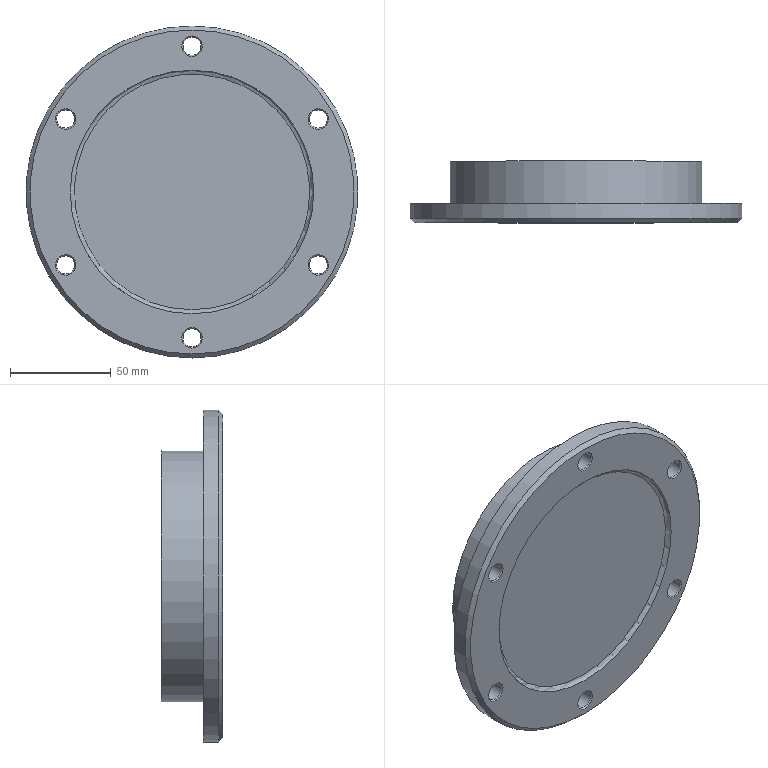Part | NX | 1 solid | 29 faces | box 165 x 30.6 x 165 mm | volume 264298 mm3 | cone 14 | cylinder 8 | plane 5 | torus 2 | commonest cylinder face diameters 9 x6 125 x1 165 x1
STEP:
#1=CARTESIAN_POINT('',(69.093,93.861,38.5));
#2=VERTEX_POINT('',#1);
#3=CARTESIAN_POINT('',(65.196,93.861,36.25));
#4=DIRECTION('',(0.,-1.,0.));
#5=DIRECTION('',(0.866,0.,0.5));
#6=AXIS2_PLACEMENT_3D('',#3,#4,#5);
#7=CIRCLE('',#6,4.5);
#8=EDGE_CURVE('',#2,#2,#7,.T.);
#9=ORIENTED_EDGE('',*,*,#8,.F.);
#10=EDGE_LOOP('',(#9));
#11=FACE_BOUND('',#10,.T.);
#12=CARTESIAN_POINT('',(69.612,93.261,38.8));
#13=VERTEX_POINT('',#12);
#14=CARTESIAN_POINT('',(65.196,93.261,36.25));
#15=DIRECTION('',(0.,1.,0.));
#16=DIRECTION('',(0.866,0.,0.5));
#17=AXIS2_PLACEMENT_3D('',#14,#15,#16);
#18=CIRCLE('',#17,5.1);
#19=EDGE_CURVE('',#13,#13,#18,.T.);
#20=ORIENTED_EDGE('',*,*,#19,.F.);
#21=EDGE_LOOP('',(#20));
#22=FACE_BOUND('',#21,.T.);
#23=CARTESIAN_POINT('',(65.196,93.261,36.25));
#24=DIRECTION('',(0.,-1.,0.));
#25=DIRECTION('',(0.866,0.,0.5));
#26=AXIS2_PLACEMENT_3D('',#23,#24,#25);
#27=CONICAL_SURFACE('',#26,5.1,45.);
#28=ADVANCED_FACE('',(#11,#22),#27,.F.);
#29=CARTESIAN_POINT('',(61.298,102.261,34.));
#30=VERTEX_POINT('',#29);
#31=CARTESIAN_POINT('',(65.196,102.261,36.25));
#32=DIRECTION('',(0.,1.,0.));
#33=DIRECTION('',(-0.866,0.,-0.5));
#34=AXIS2_PLACEMENT_3D('',#31,#32,#33);
#35=CIRCLE('',#34,4.5);
#36=EDGE_CURVE('',#30,#30,#35,.T.);
#37=ORIENTED_EDGE('',*,*,#36,.F.);
#38=EDGE_LOOP('',(#37));
#39=FACE_BOUND('',#38,.T.);
#40=CARTESIAN_POINT('',(60.779,102.861,33.7));
#41=VERTEX_POINT('',#40);
#42=CARTESIAN_POINT('',(65.196,102.861,36.25));
#43=DIRECTION('',(0.,-1.,0.));
#44=DIRECTION('',(-0.866,0.,-0.5));
#45=AXIS2_PLACEMENT_3D('',#42,#43,#44);
#46=CIRCLE('',#45,5.1);
#47=EDGE_CURVE('',#41,#41,#46,.T.);
#48=ORIENTED_EDGE('',*,*,#47,.F.);
#49=EDGE_LOOP('',(#48));
#50=FACE_BOUND('',#49,.T.);
#51=CARTESIAN_POINT('',(65.196,102.861,36.25));
#52=DIRECTION('',(0.,1.,0.));
#53=DIRECTION('',(-0.866,0.,-0.5));
#54=AXIS2_PLACEMENT_3D('',#51,#52,#53);
#55=CONICAL_SURFACE('',#54,5.1,45.);
#56=ADVANCED_FACE('',(#39,#50),#55,.F.);
#57=ORIENTED_EDGE('',*,*,#36,.T.);
#58=EDGE_LOOP('',(#57));
#59=FACE_BOUND('',#58,.T.);
#60=ORIENTED_EDGE('',*,*,#8,.T.);
#61=EDGE_LOOP('',(#60));
#62=FACE_BOUND('',#61,.T.);
#63=CARTESIAN_POINT('',(65.196,93.261,36.25));
#64=DIRECTION('',(0.,1.,0.));
#65=DIRECTION('',(-0.866,0.,-0.5));
#66=AXIS2_PLACEMENT_3D('',#63,#64,#65);
#67=CYLINDRICAL_SURFACE('',#66,4.5);
#68=ADVANCED_FACE('',(#59,#62),#67,.F.);
#69=CARTESIAN_POINT('',(69.093,93.861,-38.5));
#70=VERTEX_POINT('',#69);
#71=CARTESIAN_POINT('',(65.196,93.861,-36.25));
#72=DIRECTION('',(0.,-1.,0.));
#73=DIRECTION('',(0.866,0.,-0.5));
#74=AXIS2_PLACEMENT_3D('',#71,#72,#73);
#75=CIRCLE('',#74,4.5);
#76=EDGE_CURVE('',#70,#70,#75,.T.);
#77=ORIENTED_EDGE('',*,*,#76,.F.);
#78=EDGE_LOOP('',(#77));
#79=FACE_BOUND('',#78,.T.);
#80=CARTESIAN_POINT('',(69.612,93.261,-38.8));
#81=VERTEX_POINT('',#80);
#82=CARTESIAN_POINT('',(65.196,93.261,-36.25));
#83=DIRECTION('',(0.,1.,0.));
#84=DIRECTION('',(0.866,0.,-0.5));
#85=AXIS2_PLACEMENT_3D('',#82,#83,#84);
#86=CIRCLE('',#85,5.1);
#87=EDGE_CURVE('',#81,#81,#86,.T.);
#88=ORIENTED_EDGE('',*,*,#87,.F.);
#89=EDGE_LOOP('',(#88));
#90=FACE_BOUND('',#89,.T.);
#91=CARTESIAN_POINT('',(65.196,93.261,-36.25));
#92=DIRECTION('',(0.,-1.,0.));
#93=DIRECTION('',(0.866,0.,-0.5));
#94=AXIS2_PLACEMENT_3D('',#91,#92,#93);
#95=CONICAL_SURFACE('',#94,5.1,45.);
#96=ADVANCED_FACE('',(#79,#90),#95,.F.);
#97=CARTESIAN_POINT('',(61.298,102.261,-34.));
#98=VERTEX_POINT('',#97);
#99=CARTESIAN_POINT('',(65.196,102.261,-36.25));
#100=DIRECTION('',(0.,1.,0.));
#101=DIRECTION('',(-0.866,0.,0.5));
#102=AXIS2_PLACEMENT_3D('',#99,#100,#101);
#103=CIRCLE('',#102,4.5);
#104=EDGE_CURVE('',#98,#98,#103,.T.);
#105=ORIENTED_EDGE('',*,*,#104,.F.);
#106=EDGE_LOOP('',(#105));
#107=FACE_BOUND('',#106,.T.);
#108=CARTESIAN_POINT('',(60.779,102.861,-33.7));
#109=VERTEX_POINT('',#108);
#110=CARTESIAN_POINT('',(65.196,102.861,-36.25));
#111=DIRECTION('',(0.,-1.,0.));
#112=DIRECTION('',(-0.866,0.,0.5));
#113=AXIS2_PLACEMENT_3D('',#110,#111,#112);
#114=CIRCLE('',#113,5.1);
#115=EDGE_CURVE('',#109,#109,#114,.T.);
#116=ORIENTED_EDGE('',*,*,#115,.F.);
#117=EDGE_LOOP('',(#116));
#118=FACE_BOUND('',#117,.T.);
#119=CARTESIAN_POINT('',(65.196,102.861,-36.25));
#120=DIRECTION('',(0.,1.,0.));
#121=DIRECTION('',(-0.866,0.,0.5));
#122=AXIS2_PLACEMENT_3D('',#119,#120,#121);
#123=CONICAL_SURFACE('',#122,5.1,45.);
#124=ADVANCED_FACE('',(#107,#118),#123,.F.);
#125=ORIENTED_EDGE('',*,*,#104,.T.);
#126=EDGE_LOOP('',(#125));
#127=FACE_BOUND('',#126,.T.);
#128=ORIENTED_EDGE('',*,*,#76,.T.);
#129=EDGE_LOOP('',(#128));
#130=FACE_BOUND('',#129,.T.);
#131=CARTESIAN_POINT('',(65.196,93.261,-36.25));
#132=DIRECTION('',(0.,1.,0.));
#133=DIRECTION('',(-0.866,0.,0.5));
#134=AXIS2_PLACEMENT_3D('',#131,#132,#133);
#135=CYLINDRICAL_SURFACE('',#134,4.5);
#136=ADVANCED_FACE('',(#127,#130),#135,.F.);
#137=CARTESIAN_POINT('',(2.409,93.861,-77.));
#138=VERTEX_POINT('',#137);
#139=CARTESIAN_POINT('',(2.409,93.861,-72.5));
#140=DIRECTION('',(0.,-1.,0.));
#141=DIRECTION('',(0.,0.,-1.));
#142=AXIS2_PLACEMENT_3D('',#139,#140,#141);
#143=CIRCLE('',#142,4.5);
#144=EDGE_CURVE('',#138,#138,#143,.T.);
#145=ORIENTED_EDGE('',*,*,#144,.F.);
#146=EDGE_LOOP('',(#145));
#147=FACE_BOUND('',#146,.T.);
#148=CARTESIAN_POINT('',(2.409,93.261,-77.6));
#149=VERTEX_POINT('',#148);
#150=CARTESIAN_POINT('',(2.409,93.261,-72.5));
#151=DIRECTION('',(0.,1.,0.));
#152=DIRECTION('',(0.,0.,-1.));
#153=AXIS2_PLACEMENT_3D('',#150,#151,#152);
#154=CIRCLE('',#153,5.1);
#155=EDGE_CURVE('',#149,#149,#154,.T.);
#156=ORIENTED_EDGE('',*,*,#155,.F.);
#157=EDGE_LOOP('',(#156));
#158=FACE_BOUND('',#157,.T.);
#159=CARTESIAN_POINT('',(2.409,93.261,-72.5));
#160=DIRECTION('',(0.,-1.,0.));
#161=DIRECTION('',(0.,0.,-1.));
#162=AXIS2_PLACEMENT_3D('',#159,#160,#161);
#163=CONICAL_SURFACE('',#162,5.1,45.);
#164=ADVANCED_FACE('',(#147,#158),#163,.F.);
#165=CARTESIAN_POINT('',(2.409,102.261,-68.));
#166=VERTEX_POINT('',#165);
#167=CARTESIAN_POINT('',(2.409,102.261,-72.5));
#168=DIRECTION('',(0.,1.,0.));
#169=DIRECTION('',(0.,0.,1.));
#170=AXIS2_PLACEMENT_3D('',#167,#168,#169);
#171=CIRCLE('',#170,4.5);
#172=EDGE_CURVE('',#166,#166,#171,.T.);
#173=ORIENTED_EDGE('',*,*,#172,.F.);
#174=EDGE_LOOP('',(#173));
#175=FACE_BOUND('',#174,.T.);
#176=CARTESIAN_POINT('',(2.409,102.861,-67.4));
#177=VERTEX_POINT('',#176);
#178=CARTESIAN_POINT('',(2.409,102.861,-72.5));
#179=DIRECTION('',(0.,-1.,0.));
#180=DIRECTION('',(0.,0.,1.));
#181=AXIS2_PLACEMENT_3D('',#178,#179,#180);
#182=CIRCLE('',#181,5.1);
#183=EDGE_CURVE('',#177,#177,#182,.T.);
#184=ORIENTED_EDGE('',*,*,#183,.F.);
#185=EDGE_LOOP('',(#184));
#186=FACE_BOUND('',#185,.T.);
#187=CARTESIAN_POINT('',(2.409,102.861,-72.5));
#188=DIRECTION('',(0.,1.,0.));
#189=DIRECTION('',(0.,0.,1.));
#190=AXIS2_PLACEMENT_3D('',#187,#188,#189);
#191=CONICAL_SURFACE('',#190,5.1,45.);
#192=ADVANCED_FACE('',(#175,#186),#191,.F.);
#193=ORIENTED_EDGE('',*,*,#172,.T.);
#194=EDGE_LOOP('',(#193));
#195=FACE_BOUND('',#194,.T.);
#196=ORIENTED_EDGE('',*,*,#144,.T.);
#197=EDGE_LOOP('',(#196));
#198=FACE_BOUND('',#197,.T.);
#199=CARTESIAN_POINT('',(2.409,93.261,-72.5));
#200=DIRECTION('',(0.,1.,0.));
#201=DIRECTION('',(0.,0.,1.));
#202=AXIS2_PLACEMENT_3D('',#199,#200,#201);
#203=CYLINDRICAL_SURFACE('',#202,4.5);
#204=ADVANCED_FACE('',(#195,#198),#203,.F.);
#205=CARTESIAN_POINT('',(-64.275,93.861,-38.5));
#206=VERTEX_POINT('',#205);
#207=CARTESIAN_POINT('',(-60.378,93.861,-36.25));
#208=DIRECTION('',(0.,-1.,0.));
#209=DIRECTION('',(-0.866,0.,-0.5));
#210=AXIS2_PLACEMENT_3D('',#207,#208,#209);
#211=CIRCLE('',#210,4.5);
#212=EDGE_CURVE('',#206,#206,#211,.T.);
#213=ORIENTED_EDGE('',*,*,#212,.F.);
#214=EDGE_LOOP('',(#213));
#215=FACE_BOUND('',#214,.T.);
#216=CARTESIAN_POINT('',(-64.795,93.261,-38.8));
#217=VERTEX_POINT('',#216);
#218=CARTESIAN_POINT('',(-60.378,93.261,-36.25));
#219=DIRECTION('',(0.,1.,0.));
#220=DIRECTION('',(-0.866,0.,-0.5));
#221=AXIS2_PLACEMENT_3D('',#218,#219,#220);
#222=CIRCLE('',#221,5.1);
#223=EDGE_CURVE('',#217,#217,#222,.T.);
#224=ORIENTED_EDGE('',*,*,#223,.F.);
#225=EDGE_LOOP('',(#224));
#226=FACE_BOUND('',#225,.T.);
#227=CARTESIAN_POINT('',(-60.378,93.261,-36.25));
#228=DIRECTION('',(0.,-1.,0.));
#229=DIRECTION('',(-0.866,0.,-0.5));
#230=AXIS2_PLACEMENT_3D('',#227,#228,#229);
#231=CONICAL_SURFACE('',#230,5.1,45.);
#232=ADVANCED_FACE('',(#215,#226),#231,.F.);
#233=CARTESIAN_POINT('',(-56.481,102.261,-34.));
#234=VERTEX_POINT('',#233);
#235=CARTESIAN_POINT('',(-60.378,102.261,-36.25));
#236=DIRECTION('',(0.,1.,0.));
#237=DIRECTION('',(0.866,0.,0.5));
#238=AXIS2_PLACEMENT_3D('',#235,#236,#237);
#239=CIRCLE('',#238,4.5);
#240=EDGE_CURVE('',#234,#234,#239,.T.);
#241=ORIENTED_EDGE('',*,*,#240,.F.);
#242=EDGE_LOOP('',(#241));
#243=FACE_BOUND('',#242,.T.);
#244=CARTESIAN_POINT('',(-55.961,102.861,-33.7));
#245=VERTEX_POINT('',#244);
#246=CARTESIAN_POINT('',(-60.378,102.861,-36.25));
#247=DIRECTION('',(0.,-1.,0.));
#248=DIRECTION('',(0.866,0.,0.5));
#249=AXIS2_PLACEMENT_3D('',#246,#247,#248);
#250=CIRCLE('',#249,5.1);
#251=EDGE_CURVE('',#245,#245,#250,.T.);
#252=ORIENTED_EDGE('',*,*,#251,.F.);
#253=EDGE_LOOP('',(#252));
#254=FACE_BOUND('',#253,.T.);
#255=CARTESIAN_POINT('',(-60.378,102.861,-36.25));
#256=DIRECTION('',(0.,1.,0.));
#257=DIRECTION('',(0.866,0.,0.5));
#258=AXIS2_PLACEMENT_3D('',#255,#256,#257);
#259=CONICAL_SURFACE('',#258,5.1,45.);
#260=ADVANCED_FACE('',(#243,#254),#259,.F.);
#261=ORIENTED_EDGE('',*,*,#240,.T.);
#262=EDGE_LOOP('',(#261));
#263=FACE_BOUND('',#262,.T.);
#264=ORIENTED_EDGE('',*,*,#212,.T.);
#265=EDGE_LOOP('',(#264));
#266=FACE_BOUND('',#265,.T.);
#267=CARTESIAN_POINT('',(-60.378,93.261,-36.25));
#268=DIRECTION('',(0.,1.,0.));
#269=DIRECTION('',(0.866,0.,0.5));
#270=AXIS2_PLACEMENT_3D('',#267,#268,#269);
#271=CYLINDRICAL_SURFACE('',#270,4.5);
#272=ADVANCED_FACE('',(#263,#266),#271,.F.);
#273=CARTESIAN_POINT('',(-64.275,93.861,38.5));
#274=VERTEX_POINT('',#273);
#275=CARTESIAN_POINT('',(-60.378,93.861,36.25));
#276=DIRECTION('',(0.,-1.,0.));
#277=DIRECTION('',(-0.866,0.,0.5));
#278=AXIS2_PLACEMENT_3D('',#275,#276,#277);
#279=CIRCLE('',#278,4.5);
#280=EDGE_CURVE('',#274,#274,#279,.T.);
#281=ORIENTED_EDGE('',*,*,#280,.F.);
#282=EDGE_LOOP('',(#281));
#283=FACE_BOUND('',#282,.T.);
#284=CARTESIAN_POINT('',(-64.795,93.261,38.8));
#285=VERTEX_POINT('',#284);
#286=CARTESIAN_POINT('',(-60.378,93.261,36.25));
#287=DIRECTION('',(0.,1.,0.));
#288=DIRECTION('',(-0.866,0.,0.5));
#289=AXIS2_PLACEMENT_3D('',#286,#287,#288);
#290=CIRCLE('',#289,5.1);
#291=EDGE_CURVE('',#285,#285,#290,.T.);
#292=ORIENTED_EDGE('',*,*,#291,.F.);
#293=EDGE_LOOP('',(#292));
#294=FACE_BOUND('',#293,.T.);
#295=CARTESIAN_POINT('',(-60.378,93.261,36.25));
#296=DIRECTION('',(0.,-1.,0.));
#297=DIRECTION('',(-0.866,0.,0.5));
#298=AXIS2_PLACEMENT_3D('',#295,#296,#297);
#299=CONICAL_SURFACE('',#298,5.1,45.);
#300=ADVANCED_FACE('',(#283,#294),#299,.F.);
#301=CARTESIAN_POINT('',(-56.481,102.261,34.));
#302=VERTEX_POINT('',#301);
#303=CARTESIAN_POINT('',(-60.378,102.261,36.25));
#304=DIRECTION('',(0.,1.,0.));
#305=DIRECTION('',(0.866,0.,-0.5));
#306=AXIS2_PLACEMENT_3D('',#303,#304,#305);
#307=CIRCLE('',#306,4.5);
#308=EDGE_CURVE('',#302,#302,#307,.T.);
#309=ORIENTED_EDGE('',*,*,#308,.F.);
#310=EDGE_LOOP('',(#309));
#311=FACE_BOUND('',#310,.T.);
#312=CARTESIAN_POINT('',(-55.961,102.861,33.7));
#313=VERTEX_POINT('',#312);
#314=CARTESIAN_POINT('',(-60.378,102.861,36.25));
#315=DIRECTION('',(0.,-1.,0.));
#316=DIRECTION('',(0.866,0.,-0.5));
#317=AXIS2_PLACEMENT_3D('',#314,#315,#316);
#318=CIRCLE('',#317,5.1);
#319=EDGE_CURVE('',#313,#313,#318,.T.);
#320=ORIENTED_EDGE('',*,*,#319,.F.);
#321=EDGE_LOOP('',(#320));
#322=FACE_BOUND('',#321,.T.);
#323=CARTESIAN_POINT('',(-60.378,102.861,36.25));
#324=DIRECTION('',(0.,1.,0.));
#325=DIRECTION('',(0.866,0.,-0.5));
#326=AXIS2_PLACEMENT_3D('',#323,#324,#325);
#327=CONICAL_SURFACE('',#326,5.1,45.);
#328=ADVANCED_FACE('',(#311,#322),#327,.F.);
#329=ORIENTED_EDGE('',*,*,#308,.T.);
#330=EDGE_LOOP('',(#329));
#331=FACE_BOUND('',#330,.T.);
#332=ORIENTED_EDGE('',*,*,#280,.T.);
#333=EDGE_LOOP('',(#332));
#334=FACE_BOUND('',#333,.T.);
#335=CARTESIAN_POINT('',(-60.378,93.261,36.25));
#336=DIRECTION('',(0.,1.,0.));
#337=DIRECTION('',(0.866,0.,-0.5));
#338=AXIS2_PLACEMENT_3D('',#335,#336,#337);
#339=CYLINDRICAL_SURFACE('',#338,4.5);
#340=ADVANCED_FACE('',(#331,#334),#339,.F.);
#341=CARTESIAN_POINT('',(2.409,95.261,-58.5));
#342=VERTEX_POINT('',#341);
#343=CARTESIAN_POINT('',(2.409,95.261,0.));
#344=DIRECTION('',(0.,-1.,0.));
#345=DIRECTION('',(0.,0.,-1.));
#346=AXIS2_PLACEMENT_3D('',#343,#344,#345);
#347=CIRCLE('',#346,58.5);
#348=EDGE_CURVE('',#342,#342,#347,.T.);
#349=ORIENTED_EDGE('',*,*,#348,.T.);
#350=EDGE_LOOP('',(#349));
#351=FACE_OUTER_BOUND('',#350,.T.);
#352=CARTESIAN_POINT('',(-56.091,95.261,0.));
#353=DIRECTION('',(0.,1.,0.));
#354=DIRECTION('',(0.,0.,-1.));
#355=AXIS2_PLACEMENT_3D('',#352,#353,#354);
#356=PLANE('',#355);
#357=ADVANCED_FACE('',(#351),#356,.F.);
#358=ORIENTED_EDGE('',*,*,#348,.F.);
#359=EDGE_LOOP('',(#358));
#360=FACE_BOUND('',#359,.T.);
#361=CARTESIAN_POINT('',(2.409,93.261,-60.5));
#362=VERTEX_POINT('',#361);
#363=CARTESIAN_POINT('',(2.409,93.261,0.));
#364=DIRECTION('',(0.,-1.,0.));
#365=DIRECTION('',(0.,0.,-1.));
#366=AXIS2_PLACEMENT_3D('',#363,#364,#365);
#367=CIRCLE('',#366,60.5);
#368=EDGE_CURVE('',#362,#362,#367,.T.);
#369=ORIENTED_EDGE('',*,*,#368,.T.);
#370=EDGE_LOOP('',(#369));
#371=FACE_BOUND('',#370,.T.);
#372=CARTESIAN_POINT('',(2.409,93.261,0.));
#373=DIRECTION('',(0.,-1.,0.));
#374=DIRECTION('',(0.,0.,1.));
#375=AXIS2_PLACEMENT_3D('',#372,#373,#374);
#376=TOROIDAL_SURFACE('',#375,58.5,2.);
#377=ADVANCED_FACE('',(#360,#371),#376,.F.);
#378=ORIENTED_EDGE('',*,*,#19,.T.);
#379=EDGE_LOOP('',(#378));
#380=FACE_BOUND('',#379,.T.);
#381=ORIENTED_EDGE('',*,*,#87,.T.);
#382=EDGE_LOOP('',(#381));
#383=FACE_BOUND('',#382,.T.);
#384=ORIENTED_EDGE('',*,*,#155,.T.);
#385=EDGE_LOOP('',(#384));
#386=FACE_BOUND('',#385,.T.);
#387=ORIENTED_EDGE('',*,*,#223,.T.);
#388=EDGE_LOOP('',(#387));
#389=FACE_BOUND('',#388,.T.);
#390=ORIENTED_EDGE('',*,*,#291,.T.);
#391=EDGE_LOOP('',(#390));
#392=FACE_BOUND('',#391,.T.);
#393=CARTESIAN_POINT('',(2.409,93.261,77.6));
#394=VERTEX_POINT('',#393);
#395=CARTESIAN_POINT('',(2.409,93.261,72.5));
#396=DIRECTION('',(0.,1.,0.));
#397=DIRECTION('',(0.,0.,1.));
#398=AXIS2_PLACEMENT_3D('',#395,#396,#397);
#399=CIRCLE('',#398,5.1);
#400=EDGE_CURVE('',#394,#394,#399,.T.);
#401=ORIENTED_EDGE('',*,*,#400,.T.);
#402=EDGE_LOOP('',(#401));
#403=FACE_BOUND('',#402,.T.);
#404=ORIENTED_EDGE('',*,*,#368,.F.);
#405=EDGE_LOOP('',(#404));
#406=FACE_BOUND('',#405,.T.);
#407=CARTESIAN_POINT('',(2.409,93.261,-80.5));
#408=VERTEX_POINT('',#407);
#409=CARTESIAN_POINT('',(2.409,93.261,0.));
#410=DIRECTION('',(0.,-1.,0.));
#411=DIRECTION('',(0.,0.,-1.));
#412=AXIS2_PLACEMENT_3D('',#409,#410,#411);
#413=CIRCLE('',#412,80.5);
#414=EDGE_CURVE('',#408,#408,#413,.T.);
#415=ORIENTED_EDGE('',*,*,#414,.T.);
#416=EDGE_LOOP('',(#415));
#417=FACE_BOUND('',#416,.T.);
#418=CARTESIAN_POINT('',(-78.091,93.261,0.));
#419=DIRECTION('',(0.,1.,0.));
#420=DIRECTION('',(0.,0.,-1.));
#421=AXIS2_PLACEMENT_3D('',#418,#419,#420);
#422=PLANE('',#421);
#423=ADVANCED_FACE('',(#380,#383,#386,#389,#392,#403,#406,#417),#422,.F.);
#424=ORIENTED_EDGE('',*,*,#414,.F.);
#425=EDGE_LOOP('',(#424));
#426=FACE_BOUND('',#425,.T.);
#427=CARTESIAN_POINT('',(2.409,95.261,-82.5));
#428=VERTEX_POINT('',#427);
#429=CARTESIAN_POINT('',(2.409,95.261,0.));
#430=DIRECTION('',(0.,-1.,0.));
#431=DIRECTION('',(0.,0.,-1.));
#432=AXIS2_PLACEMENT_3D('',#429,#430,#431);
#433=CIRCLE('',#432,82.5);
#434=EDGE_CURVE('',#428,#428,#433,.T.);
#435=ORIENTED_EDGE('',*,*,#434,.T.);
#436=EDGE_LOOP('',(#435));
#437=FACE_BOUND('',#436,.T.);
#438=CARTESIAN_POINT('',(2.409,95.261,0.));
#439=DIRECTION('',(0.,1.,0.));
#440=DIRECTION('',(0.,0.,-1.));
#441=AXIS2_PLACEMENT_3D('',#438,#439,#440);
#442=CONICAL_SURFACE('',#441,82.5,45.);
#443=ADVANCED_FACE('',(#426,#437),#442,.T.);
#444=ORIENTED_EDGE('',*,*,#434,.F.);
#445=EDGE_LOOP('',(#444));
#446=FACE_BOUND('',#445,.T.);
#447=CARTESIAN_POINT('',(2.409,102.861,-82.5));
#448=VERTEX_POINT('',#447);
#449=CARTESIAN_POINT('',(2.409,102.861,0.));
#450=DIRECTION('',(0.,-1.,0.));
#451=DIRECTION('',(0.,0.,-1.));
#452=AXIS2_PLACEMENT_3D('',#449,#450,#451);
#453=CIRCLE('',#452,82.5);
#454=EDGE_CURVE('',#448,#448,#453,.T.);
#455=ORIENTED_EDGE('',*,*,#454,.T.);
#456=EDGE_LOOP('',(#455));
#457=FACE_BOUND('',#456,.T.);
#458=CARTESIAN_POINT('',(2.409,82.561,0.));
#459=DIRECTION('',(0.,-1.,0.));
#460=DIRECTION('',(0.,0.,1.));
#461=AXIS2_PLACEMENT_3D('',#458,#459,#460);
#462=CYLINDRICAL_SURFACE('',#461,82.5);
#463=ADVANCED_FACE('',(#446,#457),#462,.T.);
#464=ORIENTED_EDGE('',*,*,#47,.T.);
#465=EDGE_LOOP('',(#464));
#466=FACE_BOUND('',#465,.T.);
#467=ORIENTED_EDGE('',*,*,#115,.T.);
#468=EDGE_LOOP('',(#467));
#469=FACE_BOUND('',#468,.T.);
#470=ORIENTED_EDGE('',*,*,#183,.T.);
#471=EDGE_LOOP('',(#470));
#472=FACE_BOUND('',#471,.T.);
#473=ORIENTED_EDGE('',*,*,#251,.T.);
#474=EDGE_LOOP('',(#473));
#475=FACE_BOUND('',#474,.T.);
#476=ORIENTED_EDGE('',*,*,#319,.T.);
#477=EDGE_LOOP('',(#476));
#478=FACE_BOUND('',#477,.T.);
#479=CARTESIAN_POINT('',(2.409,102.861,67.4));
#480=VERTEX_POINT('',#479);
#481=CARTESIAN_POINT('',(2.409,102.861,72.5));
#482=DIRECTION('',(0.,-1.,0.));
#483=DIRECTION('',(0.,0.,-1.));
#484=AXIS2_PLACEMENT_3D('',#481,#482,#483);
#485=CIRCLE('',#484,5.1);
#486=EDGE_CURVE('',#480,#480,#485,.T.);
#487=ORIENTED_EDGE('',*,*,#486,.T.);
#488=EDGE_LOOP('',(#487));
#489=FACE_BOUND('',#488,.T.);
#490=ORIENTED_EDGE('',*,*,#454,.F.);
#491=EDGE_LOOP('',(#490));
#492=FACE_BOUND('',#491,.T.);
#493=CARTESIAN_POINT('',(2.409,102.861,-62.5));
#494=VERTEX_POINT('',#493);
#495=CARTESIAN_POINT('',(2.409,102.861,0.));
#496=DIRECTION('',(0.,-1.,0.));
#497=DIRECTION('',(0.,0.,-1.));
#498=AXIS2_PLACEMENT_3D('',#495,#496,#497);
#499=CIRCLE('',#498,62.5);
#500=EDGE_CURVE('',#494,#494,#499,.T.);
#501=ORIENTED_EDGE('',*,*,#500,.T.);
#502=EDGE_LOOP('',(#501));
#503=FACE_BOUND('',#502,.T.);
#504=CARTESIAN_POINT('',(-60.091,102.861,0.));
#505=DIRECTION('',(0.,-1.,0.));
#506=DIRECTION('',(0.,0.,1.));
#507=AXIS2_PLACEMENT_3D('',#504,#505,#506);
#508=PLANE('',#507);
#509=ADVANCED_FACE('',(#466,#469,#472,#475,#478,#489,#492,#503),#508,.F.);
#510=ORIENTED_EDGE('',*,*,#500,.F.);
#511=EDGE_LOOP('',(#510));
#512=FACE_BOUND('',#511,.T.);
#513=CARTESIAN_POINT('',(2.409,123.861,-62.5));
#514=VERTEX_POINT('',#513);
#515=CARTESIAN_POINT('',(2.409,123.861,0.));
#516=DIRECTION('',(0.,-1.,0.));
#517=DIRECTION('',(0.,0.,-1.));
#518=AXIS2_PLACEMENT_3D('',#515,#516,#517);
#519=CIRCLE('',#518,62.5);
#520=EDGE_CURVE('',#514,#514,#519,.T.);
#521=ORIENTED_EDGE('',*,*,#520,.T.);
#522=EDGE_LOOP('',(#521));
#523=FACE_BOUND('',#522,.T.);
#524=CARTESIAN_POINT('',(2.409,82.561,0.));
#525=DIRECTION('',(0.,-1.,0.));
#526=DIRECTION('',(0.,0.,1.));
#527=AXIS2_PLACEMENT_3D('',#524,#525,#526);
#528=CYLINDRICAL_SURFACE('',#527,62.5);
#529=ADVANCED_FACE('',(#512,#523),#528,.T.);
#530=ORIENTED_EDGE('',*,*,#520,.F.);
#531=EDGE_LOOP('',(#530));
#532=FACE_BOUND('',#531,.T.);
#533=CARTESIAN_POINT('',(2.409,123.861,-58.));
#534=VERTEX_POINT('',#533);
#535=CARTESIAN_POINT('',(2.409,123.861,0.));
#536=DIRECTION('',(0.,-1.,0.));
#537=DIRECTION('',(0.,0.,-1.));
#538=AXIS2_PLACEMENT_3D('',#535,#536,#537);
#539=CIRCLE('',#538,58.);
#540=EDGE_CURVE('',#534,#534,#539,.T.);
#541=ORIENTED_EDGE('',*,*,#540,.T.);
#542=EDGE_LOOP('',(#541));
#543=FACE_BOUND('',#542,.T.);
#544=CARTESIAN_POINT('',(-55.591,123.861,0.));
#545=DIRECTION('',(0.,-1.,0.));
#546=DIRECTION('',(0.,0.,1.));
#547=AXIS2_PLACEMENT_3D('',#544,#545,#546);
#548=PLANE('',#547);
#549=ADVANCED_FACE('',(#532,#543),#548,.F.);
#550=ORIENTED_EDGE('',*,*,#540,.F.);
#551=EDGE_LOOP('',(#550));
#552=FACE_BOUND('',#551,.T.);
#553=CARTESIAN_POINT('',(2.409,112.012,-57.408));
#554=VERTEX_POINT('',#553);
#555=CARTESIAN_POINT('',(2.409,112.012,0.));
#556=DIRECTION('',(0.,-1.,0.));
#557=DIRECTION('',(0.,0.,-1.));
#558=AXIS2_PLACEMENT_3D('',#555,#556,#557);
#559=CIRCLE('',#558,57.408);
#560=EDGE_CURVE('',#554,#554,#559,.T.);
#561=ORIENTED_EDGE('',*,*,#560,.T.);
#562=EDGE_LOOP('',(#561));
#563=FACE_BOUND('',#562,.T.);
#564=CARTESIAN_POINT('',(2.409,112.012,0.));
#565=DIRECTION('',(0.,1.,0.));
#566=DIRECTION('',(0.,0.,-1.));
#567=AXIS2_PLACEMENT_3D('',#564,#565,#566);
#568=CONICAL_SURFACE('',#567,57.408,2.862);
#569=ADVANCED_FACE('',(#552,#563),#568,.F.);
#570=ORIENTED_EDGE('',*,*,#560,.F.);
#571=EDGE_LOOP('',(#570));
#572=FACE_BOUND('',#571,.T.);
#573=CARTESIAN_POINT('',(2.409,107.261,-52.414));
#574=VERTEX_POINT('',#573);
#575=CARTESIAN_POINT('',(2.409,107.261,0.));
#576=DIRECTION('',(0.,-1.,0.));
#577=DIRECTION('',(0.,0.,-1.));
#578=AXIS2_PLACEMENT_3D('',#575,#576,#577);
#579=CIRCLE('',#578,52.414);
#580=EDGE_CURVE('',#574,#574,#579,.T.);
#581=ORIENTED_EDGE('',*,*,#580,.T.);
#582=EDGE_LOOP('',(#581));
#583=FACE_BOUND('',#582,.T.);
#584=CARTESIAN_POINT('',(2.409,112.261,0.));
#585=DIRECTION('',(0.,-1.,0.));
#586=DIRECTION('',(0.,0.,1.));
#587=AXIS2_PLACEMENT_3D('',#584,#585,#586);
#588=TOROIDAL_SURFACE('',#587,52.414,5.);
#589=ADVANCED_FACE('',(#572,#583),#588,.F.);
#590=ORIENTED_EDGE('',*,*,#580,.F.);
#591=EDGE_LOOP('',(#590));
#592=FACE_OUTER_BOUND('',#591,.T.);
#593=CARTESIAN_POINT('',(2.409,107.261,0.));
#594=DIRECTION('',(0.,-1.,0.));
#595=DIRECTION('',(0.,0.,1.));
#596=AXIS2_PLACEMENT_3D('',#593,#594,#595);
#597=PLANE('',#596);
#598=ADVANCED_FACE('',(#592),#597,.F.);
#599=CARTESIAN_POINT('',(2.409,102.261,68.));
#600=VERTEX_POINT('',#599);
#601=CARTESIAN_POINT('',(2.409,102.261,72.5));
#602=DIRECTION('',(0.,1.,0.));
#603=DIRECTION('',(0.,0.,-1.));
#604=AXIS2_PLACEMENT_3D('',#601,#602,#603);
#605=CIRCLE('',#604,4.5);
#606=EDGE_CURVE('',#600,#600,#605,.T.);
#607=ORIENTED_EDGE('',*,*,#606,.T.);
#608=EDGE_LOOP('',(#607));
#609=FACE_BOUND('',#608,.T.);
#610=CARTESIAN_POINT('',(2.409,93.861,77.));
#611=VERTEX_POINT('',#610);
#612=CARTESIAN_POINT('',(2.409,93.861,72.5));
#613=DIRECTION('',(0.,-1.,0.));
#614=DIRECTION('',(0.,0.,1.));
#615=AXIS2_PLACEMENT_3D('',#612,#613,#614);
#616=CIRCLE('',#615,4.5);
#617=EDGE_CURVE('',#611,#611,#616,.T.);
#618=ORIENTED_EDGE('',*,*,#617,.T.);
#619=EDGE_LOOP('',(#618));
#620=FACE_BOUND('',#619,.T.);
#621=CARTESIAN_POINT('',(2.409,93.261,72.5));
#622=DIRECTION('',(0.,1.,0.));
#623=DIRECTION('',(0.,0.,-1.));
#624=AXIS2_PLACEMENT_3D('',#621,#622,#623);
#625=CYLINDRICAL_SURFACE('',#624,4.5);
#626=ADVANCED_FACE('',(#609,#620),#625,.F.);
#627=ORIENTED_EDGE('',*,*,#617,.F.);
#628=EDGE_LOOP('',(#627));
#629=FACE_BOUND('',#628,.T.);
#630=ORIENTED_EDGE('',*,*,#400,.F.);
#631=EDGE_LOOP('',(#630));
#632=FACE_BOUND('',#631,.T.);
#633=CARTESIAN_POINT('',(2.409,93.261,72.5));
#634=DIRECTION('',(0.,-1.,0.));
#635=DIRECTION('',(0.,0.,1.));
#636=AXIS2_PLACEMENT_3D('',#633,#634,#635);
#637=CONICAL_SURFACE('',#636,5.1,45.);
#638=ADVANCED_FACE('',(#629,#632),#637,.F.);
#639=ORIENTED_EDGE('',*,*,#606,.F.);
#640=EDGE_LOOP('',(#639));
#641=FACE_BOUND('',#640,.T.);
#642=ORIENTED_EDGE('',*,*,#486,.F.);
#643=EDGE_LOOP('',(#642));
#644=FACE_BOUND('',#643,.T.);
#645=CARTESIAN_POINT('',(2.409,102.861,72.5));
#646=DIRECTION('',(0.,1.,0.));
#647=DIRECTION('',(0.,0.,-1.));
#648=AXIS2_PLACEMENT_3D('',#645,#646,#647);
#649=CONICAL_SURFACE('',#648,5.1,45.);
#650=ADVANCED_FACE('',(#641,#644),#649,.F.);
#651=CLOSED_SHELL('',(#28,#56,#68,#96,#124,#136,#164,#192,#204,#232,#260,#272,#300,#328,#340,#357,#377,#423,#443,#463,#509,#529,#549,#569,#589,#598,#626,#638,#650));
#652=MANIFOLD_SOLID_BREP('',#651);
#653=(LENGTH_UNIT()NAMED_UNIT(*)SI_UNIT(.MILLI.,.METRE.));
#654=UNCERTAINTY_MEASURE_WITH_UNIT(LENGTH_MEASURE(0.00002),#653,'','');
#655=(NAMED_UNIT(*)PLANE_ANGLE_UNIT()SI_UNIT($,.RADIAN.));
#656=PLANE_ANGLE_MEASURE_WITH_UNIT(PLANE_ANGLE_MEASURE(0.01745),#655);
#657=DIMENSIONAL_EXPONENTS(0.,0.,0.,0.,0.,0.,0.);
#658=(CONVERSION_BASED_UNIT('DEGREE',#656)NAMED_UNIT(#657)PLANE_ANGLE_UNIT());
#659=(NAMED_UNIT(*)SI_UNIT($,.STERADIAN.)SOLID_ANGLE_UNIT());
#660=(GEOMETRIC_REPRESENTATION_CONTEXT(3)GLOBAL_UNCERTAINTY_ASSIGNED_CONTEXT((#654))GLOBAL_UNIT_ASSIGNED_CONTEXT((#653,#658,#659))REPRESENTATION_CONTEXT('',''));
#661=ADVANCED_BREP_SHAPE_REPRESENTATION('',(#652),#660);